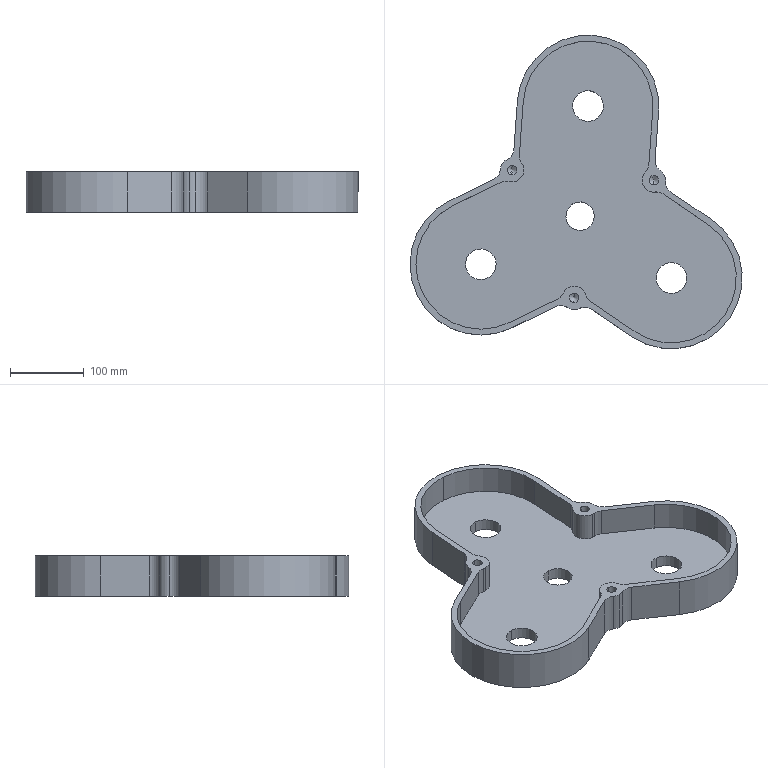Part | SolidWorks | features BaseBody 1 | 1 solid | 67 faces | box 450.446 x 425.125 x 54.4 mm | volume 2250269 mm3 | cylinder 45 | plane 16 | cone 6 | commonest cylinder face diameters 32 x21 12.8 x8 41.6 x6 176 x4 192 x4 38.4 x2